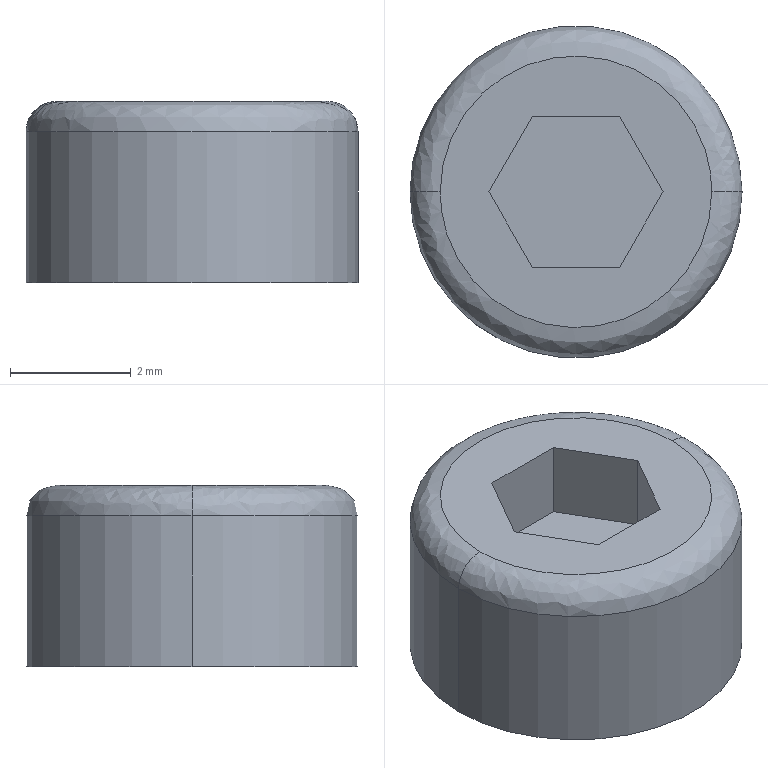Part | SolidWorks | features BaseBody 1 | 1 solid | 13 faces | box 5.5 x 5.5 x 3 mm | volume 63.35 mm3 | plane 9 | spline 2 | cylinder 2 | commonest cylinder face diameters 5.5 x2
STEP:
#1=CARTESIAN_POINT('',(-64.75,25.,20.));
#2=VERTEX_POINT('',#1);
#3=CARTESIAN_POINT('',(-70.25,25.,20.));
#4=VERTEX_POINT('',#3);
#5=CARTESIAN_POINT('',(-67.5,25.,20.));
#6=DIRECTION('',(0.,0.,-1.));
#7=DIRECTION('',(-1.,0.,0.));
#8=AXIS2_PLACEMENT_3D('',#5,#6,#7);
#9=CIRCLE('',#8,2.75);
#10=EDGE_CURVE('',#2,#4,#9,.T.);
#11=ORIENTED_EDGE('',*,*,#10,.F.);
#12=CARTESIAN_POINT('',(-65.25,25.,20.5));
#13=VERTEX_POINT('',#12);
#14=CARTESIAN_POINT('',(-65.25,25.,20.));
#15=DIRECTION('',(0.,-1.,0.));
#16=DIRECTION('',(1.,0.,0.));
#17=AXIS2_PLACEMENT_3D('',#14,#15,#16);
#18=CIRCLE('',#17,0.5);
#19=EDGE_CURVE('',#2,#13,#18,.T.);
#20=ORIENTED_EDGE('',*,*,#19,.T.);
#21=CARTESIAN_POINT('',(-69.75,25.,20.5));
#22=VERTEX_POINT('',#21);
#23=CARTESIAN_POINT('',(-65.25,25.,20.5));
#24=CARTESIAN_POINT('',(-65.25,20.5,20.5));
#25=CARTESIAN_POINT('',(-69.75,20.5,20.5));
#26=CARTESIAN_POINT('',(-69.75,25.,20.5));
#27=(BOUNDED_CURVE()B_SPLINE_CURVE(3,(#23,#24,#25,#26),.UNSPECIFIED.,.F.,.F.)B_SPLINE_CURVE_WITH_KNOTS((4,4),(0.5,1.),.UNSPECIFIED.)CURVE()GEOMETRIC_REPRESENTATION_ITEM()RATIONAL_B_SPLINE_CURVE((1.,0.3333,0.3333,1.))REPRESENTATION_ITEM(''));
#28=EDGE_CURVE('',#13,#22,#27,.T.);
#29=ORIENTED_EDGE('',*,*,#28,.T.);
#30=CARTESIAN_POINT('',(-69.75,25.,20.));
#31=DIRECTION('',(0.,1.,0.));
#32=DIRECTION('',(-1.,0.,0.));
#33=AXIS2_PLACEMENT_3D('',#30,#31,#32);
#34=CIRCLE('',#33,0.5);
#35=EDGE_CURVE('',#4,#22,#34,.T.);
#36=ORIENTED_EDGE('',*,*,#35,.F.);
#37=EDGE_LOOP('',(#11,#20,#29,#36));
#38=FACE_OUTER_BOUND('',#37,.T.);
#39=CARTESIAN_POINT('',(-64.75,25.,20.));
#40=CARTESIAN_POINT('',(-64.75,19.5,20.));
#41=CARTESIAN_POINT('',(-70.25,19.5,20.));
#42=CARTESIAN_POINT('',(-70.25,25.,20.));
#43=CARTESIAN_POINT('',(-64.75,25.,20.293));
#44=CARTESIAN_POINT('',(-64.75,19.5,20.293));
#45=CARTESIAN_POINT('',(-70.25,19.5,20.293));
#46=CARTESIAN_POINT('',(-70.25,25.,20.293));
#47=CARTESIAN_POINT('',(-64.957,25.,20.5));
#48=CARTESIAN_POINT('',(-64.957,19.914,20.5));
#49=CARTESIAN_POINT('',(-70.043,19.914,20.5));
#50=CARTESIAN_POINT('',(-70.043,25.,20.5));
#51=CARTESIAN_POINT('',(-65.25,25.,20.5));
#52=CARTESIAN_POINT('',(-65.25,20.5,20.5));
#53=CARTESIAN_POINT('',(-69.75,20.5,20.5));
#54=CARTESIAN_POINT('',(-69.75,25.,20.5));
#55=(BOUNDED_SURFACE()B_SPLINE_SURFACE(3,3,((#39,#40,#41,#42),(#43,#44,#45,#46),(#47,#48,#49,#50),(#51,#52,#53,#54)),.UNSPECIFIED.,.F.,.F.,.F.)B_SPLINE_SURFACE_WITH_KNOTS((4,4),(4,4),(0.,1.),(0.,1.),.UNSPECIFIED.)GEOMETRIC_REPRESENTATION_ITEM()RATIONAL_B_SPLINE_SURFACE(((1.,0.3333,0.3333,1.),(0.8047,0.2682,0.2682,0.8047),(0.8047,0.2682,0.2682,0.8047),(1.,0.3333,0.3333,1.)))REPRESENTATION_ITEM('')SURFACE());
#56=ADVANCED_FACE('',(#38),#55,.T.);
#57=CARTESIAN_POINT('',(-67.5,25.,20.));
#58=DIRECTION('',(0.,0.,-1.));
#59=DIRECTION('',(-1.,0.,0.));
#60=AXIS2_PLACEMENT_3D('',#57,#58,#59);
#61=CIRCLE('',#60,2.75);
#62=EDGE_CURVE('',#4,#2,#61,.T.);
#63=ORIENTED_EDGE('',*,*,#62,.T.);
#64=CARTESIAN_POINT('',(-64.75,25.,17.5));
#65=VERTEX_POINT('',#64);
#66=CARTESIAN_POINT('',(-64.75,25.,20.5));
#67=DIRECTION('',(0.,0.,-1.));
#68=VECTOR('',#67,1000.);
#69=LINE('',#66,#68);
#70=EDGE_CURVE('',#2,#65,#69,.T.);
#71=ORIENTED_EDGE('',*,*,#70,.T.);
#72=CARTESIAN_POINT('',(-70.25,25.,17.5));
#73=VERTEX_POINT('',#72);
#74=CARTESIAN_POINT('',(-67.5,25.,17.5));
#75=DIRECTION('',(0.,0.,1.));
#76=DIRECTION('',(-1.,0.,0.));
#77=AXIS2_PLACEMENT_3D('',#74,#75,#76);
#78=CIRCLE('',#77,2.75);
#79=EDGE_CURVE('',#65,#73,#78,.T.);
#80=ORIENTED_EDGE('',*,*,#79,.T.);
#81=CARTESIAN_POINT('',(-70.25,25.,20.5));
#82=DIRECTION('',(0.,0.,-1.));
#83=VECTOR('',#82,1000.);
#84=LINE('',#81,#83);
#85=EDGE_CURVE('',#4,#73,#84,.T.);
#86=ORIENTED_EDGE('',*,*,#85,.F.);
#87=EDGE_LOOP('',(#63,#71,#80,#86));
#88=FACE_OUTER_BOUND('',#87,.T.);
#89=CARTESIAN_POINT('',(-67.5,25.,20.5));
#90=DIRECTION('',(0.,0.,-1.));
#91=DIRECTION('',(-1.,0.,0.));
#92=AXIS2_PLACEMENT_3D('',#89,#90,#91);
#93=CYLINDRICAL_SURFACE('',#92,2.75);
#94=ADVANCED_FACE('',(#88),#93,.T.);
#95=ORIENTED_EDGE('',*,*,#70,.F.);
#96=ORIENTED_EDGE('',*,*,#10,.T.);
#97=ORIENTED_EDGE('',*,*,#85,.T.);
#98=CARTESIAN_POINT('',(-67.5,25.,17.5));
#99=DIRECTION('',(0.,0.,1.));
#100=DIRECTION('',(-1.,0.,0.));
#101=AXIS2_PLACEMENT_3D('',#98,#99,#100);
#102=CIRCLE('',#101,2.75);
#103=EDGE_CURVE('',#73,#65,#102,.T.);
#104=ORIENTED_EDGE('',*,*,#103,.T.);
#105=EDGE_LOOP('',(#95,#96,#97,#104));
#106=FACE_OUTER_BOUND('',#105,.T.);
#107=CARTESIAN_POINT('',(-67.5,25.,20.5));
#108=DIRECTION('',(0.,0.,-1.));
#109=DIRECTION('',(-1.,0.,0.));
#110=AXIS2_PLACEMENT_3D('',#107,#108,#109);
#111=CYLINDRICAL_SURFACE('',#110,2.75);
#112=ADVANCED_FACE('',(#106),#111,.T.);
#113=ORIENTED_EDGE('',*,*,#103,.F.);
#114=ORIENTED_EDGE('',*,*,#79,.F.);
#115=EDGE_LOOP('',(#113,#114));
#116=FACE_OUTER_BOUND('',#115,.T.);
#117=CARTESIAN_POINT('',(-67.5,25.,17.5));
#118=DIRECTION('',(0.,0.,-1.));
#119=DIRECTION('',(-1.,0.,0.));
#120=AXIS2_PLACEMENT_3D('',#117,#118,#119);
#121=PLANE('',#120);
#122=ADVANCED_FACE('',(#116),#121,.T.);
#123=ORIENTED_EDGE('',*,*,#19,.F.);
#124=ORIENTED_EDGE('',*,*,#62,.F.);
#125=ORIENTED_EDGE('',*,*,#35,.T.);
#126=CARTESIAN_POINT('',(-69.75,25.,20.5));
#127=CARTESIAN_POINT('',(-69.75,29.5,20.5));
#128=CARTESIAN_POINT('',(-65.25,29.5,20.5));
#129=CARTESIAN_POINT('',(-65.25,25.,20.5));
#130=(BOUNDED_CURVE()B_SPLINE_CURVE(3,(#126,#127,#128,#129),.UNSPECIFIED.,.F.,.F.)B_SPLINE_CURVE_WITH_KNOTS((4,4),(0.,0.5),.UNSPECIFIED.)CURVE()GEOMETRIC_REPRESENTATION_ITEM()RATIONAL_B_SPLINE_CURVE((1.,0.3333,0.3333,1.))REPRESENTATION_ITEM(''));
#131=EDGE_CURVE('',#22,#13,#130,.T.);
#132=ORIENTED_EDGE('',*,*,#131,.T.);
#133=EDGE_LOOP('',(#123,#124,#125,#132));
#134=FACE_OUTER_BOUND('',#133,.T.);
#135=CARTESIAN_POINT('',(-70.25,25.,20.));
#136=CARTESIAN_POINT('',(-70.25,30.5,20.));
#137=CARTESIAN_POINT('',(-64.75,30.5,20.));
#138=CARTESIAN_POINT('',(-64.75,25.,20.));
#139=CARTESIAN_POINT('',(-70.25,25.,20.293));
#140=CARTESIAN_POINT('',(-70.25,30.5,20.293));
#141=CARTESIAN_POINT('',(-64.75,30.5,20.293));
#142=CARTESIAN_POINT('',(-64.75,25.,20.293));
#143=CARTESIAN_POINT('',(-70.043,25.,20.5));
#144=CARTESIAN_POINT('',(-70.043,30.086,20.5));
#145=CARTESIAN_POINT('',(-64.957,30.086,20.5));
#146=CARTESIAN_POINT('',(-64.957,25.,20.5));
#147=CARTESIAN_POINT('',(-69.75,25.,20.5));
#148=CARTESIAN_POINT('',(-69.75,29.5,20.5));
#149=CARTESIAN_POINT('',(-65.25,29.5,20.5));
#150=CARTESIAN_POINT('',(-65.25,25.,20.5));
#151=(BOUNDED_SURFACE()B_SPLINE_SURFACE(3,3,((#135,#136,#137,#138),(#139,#140,#141,#142),(#143,#144,#145,#146),(#147,#148,#149,#150)),.UNSPECIFIED.,.F.,.F.,.F.)B_SPLINE_SURFACE_WITH_KNOTS((4,4),(4,4),(0.,1.),(0.,1.),.UNSPECIFIED.)GEOMETRIC_REPRESENTATION_ITEM()RATIONAL_B_SPLINE_SURFACE(((1.,0.3333,0.3333,1.),(0.8047,0.2682,0.2682,0.8047),(0.8047,0.2682,0.2682,0.8047),(1.,0.3333,0.3333,1.)))REPRESENTATION_ITEM('')SURFACE());
#152=ADVANCED_FACE('',(#134),#151,.T.);
#153=CARTESIAN_POINT('',(-66.778,23.75,20.5));
#154=VERTEX_POINT('',#153);
#155=CARTESIAN_POINT('',(-66.057,25.,20.5));
#156=VERTEX_POINT('',#155);
#157=CARTESIAN_POINT('',(-66.778,23.75,20.5));
#158=DIRECTION('',(0.5,0.866,0.));
#159=VECTOR('',#158,1000.);
#160=LINE('',#157,#159);
#161=EDGE_CURVE('',#154,#156,#160,.T.);
#162=ORIENTED_EDGE('',*,*,#161,.F.);
#163=CARTESIAN_POINT('',(-68.222,23.75,20.5));
#164=VERTEX_POINT('',#163);
#165=CARTESIAN_POINT('',(-67.5,23.75,20.5));
#166=DIRECTION('',(1.,0.,0.));
#167=VECTOR('',#166,1000.);
#168=LINE('',#165,#167);
#169=EDGE_CURVE('',#164,#154,#168,.T.);
#170=ORIENTED_EDGE('',*,*,#169,.F.);
#171=CARTESIAN_POINT('',(-68.943,25.,20.5));
#172=VERTEX_POINT('',#171);
#173=CARTESIAN_POINT('',(-68.943,25.,20.5));
#174=DIRECTION('',(0.5,-0.866,0.));
#175=VECTOR('',#174,1000.);
#176=LINE('',#173,#175);
#177=EDGE_CURVE('',#172,#164,#176,.T.);
#178=ORIENTED_EDGE('',*,*,#177,.F.);
#179=CARTESIAN_POINT('',(-68.222,26.25,20.5));
#180=VERTEX_POINT('',#179);
#181=CARTESIAN_POINT('',(-68.222,26.25,20.5));
#182=DIRECTION('',(-0.5,-0.866,0.));
#183=VECTOR('',#182,1000.);
#184=LINE('',#181,#183);
#185=EDGE_CURVE('',#180,#172,#184,.T.);
#186=ORIENTED_EDGE('',*,*,#185,.F.);
#187=CARTESIAN_POINT('',(-66.778,26.25,20.5));
#188=VERTEX_POINT('',#187);
#189=CARTESIAN_POINT('',(-67.5,26.25,20.5));
#190=DIRECTION('',(-1.,0.,0.));
#191=VECTOR('',#190,1000.);
#192=LINE('',#189,#191);
#193=EDGE_CURVE('',#188,#180,#192,.T.);
#194=ORIENTED_EDGE('',*,*,#193,.F.);
#195=CARTESIAN_POINT('',(-66.057,25.,20.5));
#196=DIRECTION('',(-0.5,0.866,0.));
#197=VECTOR('',#196,1000.);
#198=LINE('',#195,#197);
#199=EDGE_CURVE('',#156,#188,#198,.T.);
#200=ORIENTED_EDGE('',*,*,#199,.F.);
#201=EDGE_LOOP('',(#162,#170,#178,#186,#194,#200));
#202=FACE_BOUND('',#201,.T.);
#203=ORIENTED_EDGE('',*,*,#131,.F.);
#204=ORIENTED_EDGE('',*,*,#28,.F.);
#205=EDGE_LOOP('',(#203,#204));
#206=FACE_OUTER_BOUND('',#205,.T.);
#207=CARTESIAN_POINT('',(-67.5,25.,20.5));
#208=DIRECTION('',(0.,0.,-1.));
#209=DIRECTION('',(-1.,0.,0.));
#210=AXIS2_PLACEMENT_3D('',#207,#208,#209);
#211=PLANE('',#210);
#212=ADVANCED_FACE('',(#202,#206),#211,.F.);
#213=CARTESIAN_POINT('',(-66.778,26.25,19.2));
#214=VERTEX_POINT('',#213);
#215=CARTESIAN_POINT('',(-66.778,26.25,19.2));
#216=DIRECTION('',(0.,0.,1.));
#217=VECTOR('',#216,1000.);
#218=LINE('',#215,#217);
#219=EDGE_CURVE('',#214,#188,#218,.T.);
#220=ORIENTED_EDGE('',*,*,#219,.F.);
#221=CARTESIAN_POINT('',(-66.057,25.,19.2));
#222=VERTEX_POINT('',#221);
#223=CARTESIAN_POINT('',(-66.057,25.,19.2));
#224=DIRECTION('',(-0.5,0.866,0.));
#225=VECTOR('',#224,1000.);
#226=LINE('',#223,#225);
#227=EDGE_CURVE('',#222,#214,#226,.T.);
#228=ORIENTED_EDGE('',*,*,#227,.F.);
#229=CARTESIAN_POINT('',(-66.057,25.,19.2));
#230=DIRECTION('',(0.,0.,-1.));
#231=VECTOR('',#230,1000.);
#232=LINE('',#229,#231);
#233=EDGE_CURVE('',#156,#222,#232,.T.);
#234=ORIENTED_EDGE('',*,*,#233,.F.);
#235=ORIENTED_EDGE('',*,*,#199,.T.);
#236=EDGE_LOOP('',(#220,#228,#234,#235));
#237=FACE_OUTER_BOUND('',#236,.T.);
#238=CARTESIAN_POINT('',(-66.057,25.,19.2));
#239=DIRECTION('',(0.866,0.5,0.));
#240=DIRECTION('',(-0.5,0.866,0.));
#241=AXIS2_PLACEMENT_3D('',#238,#239,#240);
#242=PLANE('',#241);
#243=ADVANCED_FACE('',(#237),#242,.F.);
#244=ORIENTED_EDGE('',*,*,#233,.T.);
#245=CARTESIAN_POINT('',(-66.778,23.75,19.2));
#246=VERTEX_POINT('',#245);
#247=CARTESIAN_POINT('',(-66.778,23.75,19.2));
#248=DIRECTION('',(0.5,0.866,0.));
#249=VECTOR('',#248,1000.);
#250=LINE('',#247,#249);
#251=EDGE_CURVE('',#246,#222,#250,.T.);
#252=ORIENTED_EDGE('',*,*,#251,.F.);
#253=CARTESIAN_POINT('',(-66.778,23.75,19.2));
#254=DIRECTION('',(0.,0.,-1.));
#255=VECTOR('',#254,1000.);
#256=LINE('',#253,#255);
#257=EDGE_CURVE('',#154,#246,#256,.T.);
#258=ORIENTED_EDGE('',*,*,#257,.F.);
#259=ORIENTED_EDGE('',*,*,#161,.T.);
#260=EDGE_LOOP('',(#244,#252,#258,#259));
#261=FACE_OUTER_BOUND('',#260,.T.);
#262=CARTESIAN_POINT('',(-66.778,23.75,19.2));
#263=DIRECTION('',(0.866,-0.5,0.));
#264=DIRECTION('',(0.5,0.866,0.));
#265=AXIS2_PLACEMENT_3D('',#262,#263,#264);
#266=PLANE('',#265);
#267=ADVANCED_FACE('',(#261),#266,.F.);
#268=ORIENTED_EDGE('',*,*,#257,.T.);
#269=CARTESIAN_POINT('',(-68.222,23.75,19.2));
#270=VERTEX_POINT('',#269);
#271=CARTESIAN_POINT('',(-68.222,23.75,19.2));
#272=DIRECTION('',(1.,0.,0.));
#273=VECTOR('',#272,1000.);
#274=LINE('',#271,#273);
#275=EDGE_CURVE('',#270,#246,#274,.T.);
#276=ORIENTED_EDGE('',*,*,#275,.F.);
#277=CARTESIAN_POINT('',(-68.222,23.75,19.2));
#278=DIRECTION('',(0.,0.,-1.));
#279=VECTOR('',#278,1000.);
#280=LINE('',#277,#279);
#281=EDGE_CURVE('',#164,#270,#280,.T.);
#282=ORIENTED_EDGE('',*,*,#281,.F.);
#283=ORIENTED_EDGE('',*,*,#169,.T.);
#284=EDGE_LOOP('',(#268,#276,#282,#283));
#285=FACE_OUTER_BOUND('',#284,.T.);
#286=CARTESIAN_POINT('',(-68.222,23.75,19.2));
#287=DIRECTION('',(0.,-1.,0.));
#288=DIRECTION('',(0.,0.,-1.));
#289=AXIS2_PLACEMENT_3D('',#286,#287,#288);
#290=PLANE('',#289);
#291=ADVANCED_FACE('',(#285),#290,.F.);
#292=ORIENTED_EDGE('',*,*,#281,.T.);
#293=CARTESIAN_POINT('',(-68.943,25.,19.2));
#294=VERTEX_POINT('',#293);
#295=CARTESIAN_POINT('',(-68.943,25.,19.2));
#296=DIRECTION('',(0.5,-0.866,0.));
#297=VECTOR('',#296,1000.);
#298=LINE('',#295,#297);
#299=EDGE_CURVE('',#294,#270,#298,.T.);
#300=ORIENTED_EDGE('',*,*,#299,.F.);
#301=CARTESIAN_POINT('',(-68.943,25.,19.2));
#302=DIRECTION('',(0.,0.,-1.));
#303=VECTOR('',#302,1000.);
#304=LINE('',#301,#303);
#305=EDGE_CURVE('',#172,#294,#304,.T.);
#306=ORIENTED_EDGE('',*,*,#305,.F.);
#307=ORIENTED_EDGE('',*,*,#177,.T.);
#308=EDGE_LOOP('',(#292,#300,#306,#307));
#309=FACE_OUTER_BOUND('',#308,.T.);
#310=CARTESIAN_POINT('',(-68.943,25.,19.2));
#311=DIRECTION('',(-0.866,-0.5,0.));
#312=DIRECTION('',(0.5,-0.866,0.));
#313=AXIS2_PLACEMENT_3D('',#310,#311,#312);
#314=PLANE('',#313);
#315=ADVANCED_FACE('',(#309),#314,.F.);
#316=ORIENTED_EDGE('',*,*,#305,.T.);
#317=CARTESIAN_POINT('',(-68.222,26.25,19.2));
#318=VERTEX_POINT('',#317);
#319=CARTESIAN_POINT('',(-68.222,26.25,19.2));
#320=DIRECTION('',(-0.5,-0.866,0.));
#321=VECTOR('',#320,1000.);
#322=LINE('',#319,#321);
#323=EDGE_CURVE('',#318,#294,#322,.T.);
#324=ORIENTED_EDGE('',*,*,#323,.F.);
#325=CARTESIAN_POINT('',(-68.222,26.25,19.2));
#326=DIRECTION('',(0.,0.,-1.));
#327=VECTOR('',#326,1000.);
#328=LINE('',#325,#327);
#329=EDGE_CURVE('',#180,#318,#328,.T.);
#330=ORIENTED_EDGE('',*,*,#329,.F.);
#331=ORIENTED_EDGE('',*,*,#185,.T.);
#332=EDGE_LOOP('',(#316,#324,#330,#331));
#333=FACE_OUTER_BOUND('',#332,.T.);
#334=CARTESIAN_POINT('',(-68.222,26.25,19.2));
#335=DIRECTION('',(-0.866,0.5,0.));
#336=DIRECTION('',(-0.5,-0.866,0.));
#337=AXIS2_PLACEMENT_3D('',#334,#335,#336);
#338=PLANE('',#337);
#339=ADVANCED_FACE('',(#333),#338,.F.);
#340=ORIENTED_EDGE('',*,*,#329,.T.);
#341=CARTESIAN_POINT('',(-66.778,26.25,19.2));
#342=DIRECTION('',(-1.,0.,0.));
#343=VECTOR('',#342,1000.);
#344=LINE('',#341,#343);
#345=EDGE_CURVE('',#214,#318,#344,.T.);
#346=ORIENTED_EDGE('',*,*,#345,.F.);
#347=ORIENTED_EDGE('',*,*,#219,.T.);
#348=ORIENTED_EDGE('',*,*,#193,.T.);
#349=EDGE_LOOP('',(#340,#346,#347,#348));
#350=FACE_OUTER_BOUND('',#349,.T.);
#351=CARTESIAN_POINT('',(-66.778,26.25,19.2));
#352=DIRECTION('',(0.,1.,0.));
#353=DIRECTION('',(0.,0.,1.));
#354=AXIS2_PLACEMENT_3D('',#351,#352,#353);
#355=PLANE('',#354);
#356=ADVANCED_FACE('',(#350),#355,.F.);
#357=ORIENTED_EDGE('',*,*,#299,.T.);
#358=ORIENTED_EDGE('',*,*,#275,.T.);
#359=ORIENTED_EDGE('',*,*,#251,.T.);
#360=ORIENTED_EDGE('',*,*,#227,.T.);
#361=ORIENTED_EDGE('',*,*,#345,.T.);
#362=ORIENTED_EDGE('',*,*,#323,.T.);
#363=EDGE_LOOP('',(#357,#358,#359,#360,#361,#362));
#364=FACE_OUTER_BOUND('',#363,.T.);
#365=CARTESIAN_POINT('',(0.,0.,19.2));
#366=DIRECTION('',(0.,0.,1.));
#367=DIRECTION('',(1.,0.,0.));
#368=AXIS2_PLACEMENT_3D('',#365,#366,#367);
#369=PLANE('',#368);
#370=ADVANCED_FACE('',(#364),#369,.T.);
#371=CLOSED_SHELL('',(#56,#94,#112,#122,#152,#212,#243,#267,#291,#315,#339,#356,#370));
#372=MANIFOLD_SOLID_BREP('',#371);
#373=CARTESIAN_POINT('',(0.,0.,0.));
#374=DIRECTION('',(0.,0.,1.));
#375=DIRECTION('',(1.,0.,0.));
#376=AXIS2_PLACEMENT_3D('',#373,#374,#375);
#377=(LENGTH_UNIT()NAMED_UNIT(*)SI_UNIT(.MILLI.,.METRE.));
#378=UNCERTAINTY_MEASURE_WITH_UNIT(LENGTH_MEASURE(0.00001),#377,'','');
#379=(NAMED_UNIT(*)PLANE_ANGLE_UNIT()SI_UNIT($,.RADIAN.));
#380=(NAMED_UNIT(*)SI_UNIT($,.STERADIAN.)SOLID_ANGLE_UNIT());
#381=(GEOMETRIC_REPRESENTATION_CONTEXT(3)GLOBAL_UNCERTAINTY_ASSIGNED_CONTEXT((#378))GLOBAL_UNIT_ASSIGNED_CONTEXT((#377,#379,#380))REPRESENTATION_CONTEXT('',''));
#382=ADVANCED_BREP_SHAPE_REPRESENTATION('',(#372,#376),#381);